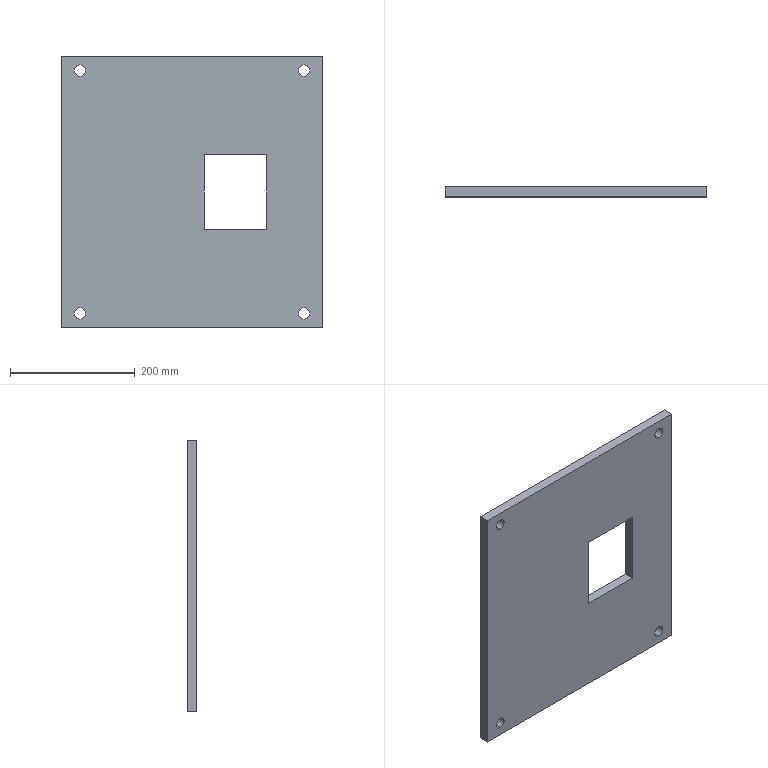Part | STEP file | 01-Base plate 1 | 1 solid | 18 faces | box 420 x 16 x 435 mm | volume 2714914 mm3 | plane 10 | cylinder 8 | commonest cylinder face diameters 18 x8
STEP:
#1=CARTESIAN_POINT('',(0.,0.,0.));
#2=DIRECTION('',(0.,0.,1.));
#3=DIRECTION('',(1.,0.,0.));
#4=AXIS2_PLACEMENT_3D('',#1,#2,#3);
#5=CARTESIAN_POINT('',(30.,0.,421.5));
#6=VERTEX_POINT('',#5);
#7=CARTESIAN_POINT('',(30.,16.,421.5));
#8=VERTEX_POINT('',#7);
#9=CARTESIAN_POINT('',(30.,-14.,421.5));
#10=DIRECTION('',(0.,1.,0.));
#11=VECTOR('',#10,1.);
#12=LINE('',#9,#11);
#13=CARTESIAN_POINT('',(30.,-14.,412.5));
#14=DIRECTION('',(0.,1.,0.));
#15=DIRECTION('',(0.,0.,1.));
#16=AXIS2_PLACEMENT_3D('',#13,#14,#15);
#17=CYLINDRICAL_SURFACE('',#16,9.);
#18=CARTESIAN_POINT('',(6.283,0.));
#19=DIRECTION('',(0.,1.));
#20=VECTOR('',#19,1.);
#21=LINE('',#18,#20);
#22=(GEOMETRIC_REPRESENTATION_CONTEXT(2)PARAMETRIC_REPRESENTATION_CONTEXT()REPRESENTATION_CONTEXT('',''));
#23=DEFINITIONAL_REPRESENTATION('',(#21),#22);
#24=PCURVE('',#17,#23);
#25=CARTESIAN_POINT('',(30.,-14.,412.5));
#26=DIRECTION('',(0.,1.,0.));
#27=DIRECTION('',(0.,0.,1.));
#28=AXIS2_PLACEMENT_3D('',#25,#26,#27);
#29=CYLINDRICAL_SURFACE('',#28,9.);
#30=CARTESIAN_POINT('',(0.,0.));
#31=DIRECTION('',(0.,1.));
#32=VECTOR('',#31,1.);
#33=LINE('',#30,#32);
#34=(GEOMETRIC_REPRESENTATION_CONTEXT(2)PARAMETRIC_REPRESENTATION_CONTEXT()REPRESENTATION_CONTEXT('',''));
#35=DEFINITIONAL_REPRESENTATION('',(#33),#34);
#36=PCURVE('',#29,#35);
#37=SURFACE_CURVE('',#12,(#24,#36),.PCURVE_S1.);
#38=EDGE_CURVE('',#6,#8,#37,.T.);
#39=ORIENTED_EDGE('',*,*,#38,.T.);
#40=CARTESIAN_POINT('',(30.,16.,403.5));
#41=VERTEX_POINT('',#40);
#42=CARTESIAN_POINT('',(30.,16.,412.5));
#43=DIRECTION('',(0.,1.,0.));
#44=DIRECTION('',(0.,0.,1.));
#45=AXIS2_PLACEMENT_3D('',#42,#43,#44);
#46=CIRCLE('',#45,9.);
#47=CARTESIAN_POINT('',(0.,30.));
#48=DIRECTION('',(1.,0.));
#49=VECTOR('',#48,1.);
#50=LINE('',#47,#49);
#51=(GEOMETRIC_REPRESENTATION_CONTEXT(2)PARAMETRIC_REPRESENTATION_CONTEXT()REPRESENTATION_CONTEXT('',''));
#52=DEFINITIONAL_REPRESENTATION('',(#50),#51);
#53=PCURVE('',#17,#52);
#54=CARTESIAN_POINT('',(0.,16.,0.));
#55=DIRECTION('',(0.,1.,0.));
#56=DIRECTION('',(0.,0.,1.));
#57=AXIS2_PLACEMENT_3D('',#54,#55,#56);
#58=PLANE('',#57);
#59=CARTESIAN_POINT('',(412.5,30.));
#60=DIRECTION('',(1.,0.));
#61=AXIS2_PLACEMENT_2D('',#59,#60);
#62=CIRCLE('',#61,9.);
#63=(GEOMETRIC_REPRESENTATION_CONTEXT(2)PARAMETRIC_REPRESENTATION_CONTEXT()REPRESENTATION_CONTEXT('',''));
#64=DEFINITIONAL_REPRESENTATION('',(#62),#63);
#65=PCURVE('',#58,#64);
#66=SURFACE_CURVE('',#46,(#53,#65),.PCURVE_S1.);
#67=EDGE_CURVE('',#41,#8,#66,.T.);
#68=ORIENTED_EDGE('',*,*,#67,.F.);
#69=CARTESIAN_POINT('',(30.,0.,403.5));
#70=VERTEX_POINT('',#69);
#71=CARTESIAN_POINT('',(30.,-14.,403.5));
#72=DIRECTION('',(0.,1.,0.));
#73=VECTOR('',#72,1.);
#74=LINE('',#71,#73);
#75=CARTESIAN_POINT('',(3.142,0.));
#76=DIRECTION('',(0.,1.));
#77=VECTOR('',#76,1.);
#78=LINE('',#75,#77);
#79=(GEOMETRIC_REPRESENTATION_CONTEXT(2)PARAMETRIC_REPRESENTATION_CONTEXT()REPRESENTATION_CONTEXT('',''));
#80=DEFINITIONAL_REPRESENTATION('',(#78),#79);
#81=PCURVE('',#17,#80);
#82=CARTESIAN_POINT('',(3.142,0.));
#83=DIRECTION('',(0.,1.));
#84=VECTOR('',#83,1.);
#85=LINE('',#82,#84);
#86=(GEOMETRIC_REPRESENTATION_CONTEXT(2)PARAMETRIC_REPRESENTATION_CONTEXT()REPRESENTATION_CONTEXT('',''));
#87=DEFINITIONAL_REPRESENTATION('',(#85),#86);
#88=PCURVE('',#29,#87);
#89=SURFACE_CURVE('',#74,(#81,#88),.PCURVE_S1.);
#90=EDGE_CURVE('',#70,#41,#89,.T.);
#91=ORIENTED_EDGE('',*,*,#90,.F.);
#92=CARTESIAN_POINT('',(30.,0.,412.5));
#93=DIRECTION('',(0.,1.,0.));
#94=DIRECTION('',(0.,0.,1.));
#95=AXIS2_PLACEMENT_3D('',#92,#93,#94);
#96=CIRCLE('',#95,9.);
#97=CARTESIAN_POINT('',(0.,14.));
#98=DIRECTION('',(1.,0.));
#99=VECTOR('',#98,1.);
#100=LINE('',#97,#99);
#101=(GEOMETRIC_REPRESENTATION_CONTEXT(2)PARAMETRIC_REPRESENTATION_CONTEXT()REPRESENTATION_CONTEXT('',''));
#102=DEFINITIONAL_REPRESENTATION('',(#100),#101);
#103=PCURVE('',#17,#102);
#104=CARTESIAN_POINT('',(0.,0.,0.));
#105=DIRECTION('',(0.,1.,0.));
#106=DIRECTION('',(0.,0.,1.));
#107=AXIS2_PLACEMENT_3D('',#104,#105,#106);
#108=PLANE('',#107);
#109=CARTESIAN_POINT('',(412.5,30.));
#110=DIRECTION('',(1.,0.));
#111=AXIS2_PLACEMENT_2D('',#109,#110);
#112=CIRCLE('',#111,9.);
#113=(GEOMETRIC_REPRESENTATION_CONTEXT(2)PARAMETRIC_REPRESENTATION_CONTEXT()REPRESENTATION_CONTEXT('',''));
#114=DEFINITIONAL_REPRESENTATION('',(#112),#113);
#115=PCURVE('',#108,#114);
#116=SURFACE_CURVE('',#96,(#103,#115),.PCURVE_S1.);
#117=EDGE_CURVE('',#70,#6,#116,.T.);
#118=ORIENTED_EDGE('',*,*,#117,.T.);
#119=EDGE_LOOP('',(#39,#68,#91,#118));
#120=FACE_BOUND('',#119,.F.);
#121=ADVANCED_FACE('',(#120),#17,.F.);
#122=CARTESIAN_POINT('',(390.,0.,421.5));
#123=VERTEX_POINT('',#122);
#124=CARTESIAN_POINT('',(390.,16.,421.5));
#125=VERTEX_POINT('',#124);
#126=CARTESIAN_POINT('',(390.,-14.,421.5));
#127=DIRECTION('',(0.,1.,0.));
#128=VECTOR('',#127,1.);
#129=LINE('',#126,#128);
#130=CARTESIAN_POINT('',(390.,-14.,412.5));
#131=DIRECTION('',(0.,1.,0.));
#132=DIRECTION('',(0.,0.,1.));
#133=AXIS2_PLACEMENT_3D('',#130,#131,#132);
#134=CYLINDRICAL_SURFACE('',#133,9.);
#135=CARTESIAN_POINT('',(6.283,0.));
#136=DIRECTION('',(0.,1.));
#137=VECTOR('',#136,1.);
#138=LINE('',#135,#137);
#139=(GEOMETRIC_REPRESENTATION_CONTEXT(2)PARAMETRIC_REPRESENTATION_CONTEXT()REPRESENTATION_CONTEXT('',''));
#140=DEFINITIONAL_REPRESENTATION('',(#138),#139);
#141=PCURVE('',#134,#140);
#142=CARTESIAN_POINT('',(390.,-14.,412.5));
#143=DIRECTION('',(0.,1.,0.));
#144=DIRECTION('',(0.,0.,1.));
#145=AXIS2_PLACEMENT_3D('',#142,#143,#144);
#146=CYLINDRICAL_SURFACE('',#145,9.);
#147=CARTESIAN_POINT('',(0.,0.));
#148=DIRECTION('',(0.,1.));
#149=VECTOR('',#148,1.);
#150=LINE('',#147,#149);
#151=(GEOMETRIC_REPRESENTATION_CONTEXT(2)PARAMETRIC_REPRESENTATION_CONTEXT()REPRESENTATION_CONTEXT('',''));
#152=DEFINITIONAL_REPRESENTATION('',(#150),#151);
#153=PCURVE('',#146,#152);
#154=SURFACE_CURVE('',#129,(#141,#153),.PCURVE_S1.);
#155=EDGE_CURVE('',#123,#125,#154,.T.);
#156=ORIENTED_EDGE('',*,*,#155,.T.);
#157=CARTESIAN_POINT('',(390.,16.,403.5));
#158=VERTEX_POINT('',#157);
#159=CARTESIAN_POINT('',(390.,16.,412.5));
#160=DIRECTION('',(0.,1.,0.));
#161=DIRECTION('',(0.,0.,1.));
#162=AXIS2_PLACEMENT_3D('',#159,#160,#161);
#163=CIRCLE('',#162,9.);
#164=CARTESIAN_POINT('',(0.,30.));
#165=DIRECTION('',(1.,0.));
#166=VECTOR('',#165,1.);
#167=LINE('',#164,#166);
#168=(GEOMETRIC_REPRESENTATION_CONTEXT(2)PARAMETRIC_REPRESENTATION_CONTEXT()REPRESENTATION_CONTEXT('',''));
#169=DEFINITIONAL_REPRESENTATION('',(#167),#168);
#170=PCURVE('',#134,#169);
#171=CARTESIAN_POINT('',(412.5,390.));
#172=DIRECTION('',(1.,0.));
#173=AXIS2_PLACEMENT_2D('',#171,#172);
#174=CIRCLE('',#173,9.);
#175=(GEOMETRIC_REPRESENTATION_CONTEXT(2)PARAMETRIC_REPRESENTATION_CONTEXT()REPRESENTATION_CONTEXT('',''));
#176=DEFINITIONAL_REPRESENTATION('',(#174),#175);
#177=PCURVE('',#58,#176);
#178=SURFACE_CURVE('',#163,(#170,#177),.PCURVE_S1.);
#179=EDGE_CURVE('',#158,#125,#178,.T.);
#180=ORIENTED_EDGE('',*,*,#179,.F.);
#181=CARTESIAN_POINT('',(390.,0.,403.5));
#182=VERTEX_POINT('',#181);
#183=CARTESIAN_POINT('',(390.,-14.,403.5));
#184=DIRECTION('',(0.,1.,0.));
#185=VECTOR('',#184,1.);
#186=LINE('',#183,#185);
#187=CARTESIAN_POINT('',(3.142,0.));
#188=DIRECTION('',(0.,1.));
#189=VECTOR('',#188,1.);
#190=LINE('',#187,#189);
#191=(GEOMETRIC_REPRESENTATION_CONTEXT(2)PARAMETRIC_REPRESENTATION_CONTEXT()REPRESENTATION_CONTEXT('',''));
#192=DEFINITIONAL_REPRESENTATION('',(#190),#191);
#193=PCURVE('',#134,#192);
#194=CARTESIAN_POINT('',(3.142,0.));
#195=DIRECTION('',(0.,1.));
#196=VECTOR('',#195,1.);
#197=LINE('',#194,#196);
#198=(GEOMETRIC_REPRESENTATION_CONTEXT(2)PARAMETRIC_REPRESENTATION_CONTEXT()REPRESENTATION_CONTEXT('',''));
#199=DEFINITIONAL_REPRESENTATION('',(#197),#198);
#200=PCURVE('',#146,#199);
#201=SURFACE_CURVE('',#186,(#193,#200),.PCURVE_S1.);
#202=EDGE_CURVE('',#182,#158,#201,.T.);
#203=ORIENTED_EDGE('',*,*,#202,.F.);
#204=CARTESIAN_POINT('',(390.,0.,412.5));
#205=DIRECTION('',(0.,1.,0.));
#206=DIRECTION('',(0.,0.,1.));
#207=AXIS2_PLACEMENT_3D('',#204,#205,#206);
#208=CIRCLE('',#207,9.);
#209=CARTESIAN_POINT('',(0.,14.));
#210=DIRECTION('',(1.,0.));
#211=VECTOR('',#210,1.);
#212=LINE('',#209,#211);
#213=(GEOMETRIC_REPRESENTATION_CONTEXT(2)PARAMETRIC_REPRESENTATION_CONTEXT()REPRESENTATION_CONTEXT('',''));
#214=DEFINITIONAL_REPRESENTATION('',(#212),#213);
#215=PCURVE('',#134,#214);
#216=CARTESIAN_POINT('',(412.5,390.));
#217=DIRECTION('',(1.,0.));
#218=AXIS2_PLACEMENT_2D('',#216,#217);
#219=CIRCLE('',#218,9.);
#220=(GEOMETRIC_REPRESENTATION_CONTEXT(2)PARAMETRIC_REPRESENTATION_CONTEXT()REPRESENTATION_CONTEXT('',''));
#221=DEFINITIONAL_REPRESENTATION('',(#219),#220);
#222=PCURVE('',#108,#221);
#223=SURFACE_CURVE('',#208,(#215,#222),.PCURVE_S1.);
#224=EDGE_CURVE('',#182,#123,#223,.T.);
#225=ORIENTED_EDGE('',*,*,#224,.T.);
#226=EDGE_LOOP('',(#156,#180,#203,#225));
#227=FACE_BOUND('',#226,.F.);
#228=ADVANCED_FACE('',(#227),#134,.F.);
#229=CARTESIAN_POINT('',(390.,0.,31.5));
#230=VERTEX_POINT('',#229);
#231=CARTESIAN_POINT('',(390.,16.,31.5));
#232=VERTEX_POINT('',#231);
#233=CARTESIAN_POINT('',(390.,-14.,31.5));
#234=DIRECTION('',(0.,1.,0.));
#235=VECTOR('',#234,1.);
#236=LINE('',#233,#235);
#237=CARTESIAN_POINT('',(390.,-14.,22.5));
#238=DIRECTION('',(0.,1.,0.));
#239=DIRECTION('',(0.,0.,1.));
#240=AXIS2_PLACEMENT_3D('',#237,#238,#239);
#241=CYLINDRICAL_SURFACE('',#240,9.);
#242=CARTESIAN_POINT('',(6.283,0.));
#243=DIRECTION('',(0.,1.));
#244=VECTOR('',#243,1.);
#245=LINE('',#242,#244);
#246=(GEOMETRIC_REPRESENTATION_CONTEXT(2)PARAMETRIC_REPRESENTATION_CONTEXT()REPRESENTATION_CONTEXT('',''));
#247=DEFINITIONAL_REPRESENTATION('',(#245),#246);
#248=PCURVE('',#241,#247);
#249=CARTESIAN_POINT('',(390.,-14.,22.5));
#250=DIRECTION('',(0.,1.,0.));
#251=DIRECTION('',(0.,0.,1.));
#252=AXIS2_PLACEMENT_3D('',#249,#250,#251);
#253=CYLINDRICAL_SURFACE('',#252,9.);
#254=CARTESIAN_POINT('',(0.,0.));
#255=DIRECTION('',(0.,1.));
#256=VECTOR('',#255,1.);
#257=LINE('',#254,#256);
#258=(GEOMETRIC_REPRESENTATION_CONTEXT(2)PARAMETRIC_REPRESENTATION_CONTEXT()REPRESENTATION_CONTEXT('',''));
#259=DEFINITIONAL_REPRESENTATION('',(#257),#258);
#260=PCURVE('',#253,#259);
#261=SURFACE_CURVE('',#236,(#248,#260),.PCURVE_S1.);
#262=EDGE_CURVE('',#230,#232,#261,.T.);
#263=ORIENTED_EDGE('',*,*,#262,.T.);
#264=CARTESIAN_POINT('',(390.,16.,13.5));
#265=VERTEX_POINT('',#264);
#266=CARTESIAN_POINT('',(390.,16.,22.5));
#267=DIRECTION('',(0.,1.,0.));
#268=DIRECTION('',(0.,0.,1.));
#269=AXIS2_PLACEMENT_3D('',#266,#267,#268);
#270=CIRCLE('',#269,9.);
#271=CARTESIAN_POINT('',(0.,30.));
#272=DIRECTION('',(1.,0.));
#273=VECTOR('',#272,1.);
#274=LINE('',#271,#273);
#275=(GEOMETRIC_REPRESENTATION_CONTEXT(2)PARAMETRIC_REPRESENTATION_CONTEXT()REPRESENTATION_CONTEXT('',''));
#276=DEFINITIONAL_REPRESENTATION('',(#274),#275);
#277=PCURVE('',#241,#276);
#278=CARTESIAN_POINT('',(22.5,390.));
#279=DIRECTION('',(1.,0.));
#280=AXIS2_PLACEMENT_2D('',#278,#279);
#281=CIRCLE('',#280,9.);
#282=(GEOMETRIC_REPRESENTATION_CONTEXT(2)PARAMETRIC_REPRESENTATION_CONTEXT()REPRESENTATION_CONTEXT('',''));
#283=DEFINITIONAL_REPRESENTATION('',(#281),#282);
#284=PCURVE('',#58,#283);
#285=SURFACE_CURVE('',#270,(#277,#284),.PCURVE_S1.);
#286=EDGE_CURVE('',#265,#232,#285,.T.);
#287=ORIENTED_EDGE('',*,*,#286,.F.);
#288=CARTESIAN_POINT('',(390.,0.,13.5));
#289=VERTEX_POINT('',#288);
#290=CARTESIAN_POINT('',(390.,-14.,13.5));
#291=DIRECTION('',(0.,1.,0.));
#292=VECTOR('',#291,1.);
#293=LINE('',#290,#292);
#294=CARTESIAN_POINT('',(3.142,0.));
#295=DIRECTION('',(0.,1.));
#296=VECTOR('',#295,1.);
#297=LINE('',#294,#296);
#298=(GEOMETRIC_REPRESENTATION_CONTEXT(2)PARAMETRIC_REPRESENTATION_CONTEXT()REPRESENTATION_CONTEXT('',''));
#299=DEFINITIONAL_REPRESENTATION('',(#297),#298);
#300=PCURVE('',#241,#299);
#301=CARTESIAN_POINT('',(3.142,0.));
#302=DIRECTION('',(0.,1.));
#303=VECTOR('',#302,1.);
#304=LINE('',#301,#303);
#305=(GEOMETRIC_REPRESENTATION_CONTEXT(2)PARAMETRIC_REPRESENTATION_CONTEXT()REPRESENTATION_CONTEXT('',''));
#306=DEFINITIONAL_REPRESENTATION('',(#304),#305);
#307=PCURVE('',#253,#306);
#308=SURFACE_CURVE('',#293,(#300,#307),.PCURVE_S1.);
#309=EDGE_CURVE('',#289,#265,#308,.T.);
#310=ORIENTED_EDGE('',*,*,#309,.F.);
#311=CARTESIAN_POINT('',(390.,0.,22.5));
#312=DIRECTION('',(0.,1.,0.));
#313=DIRECTION('',(0.,0.,1.));
#314=AXIS2_PLACEMENT_3D('',#311,#312,#313);
#315=CIRCLE('',#314,9.);
#316=CARTESIAN_POINT('',(0.,14.));
#317=DIRECTION('',(1.,0.));
#318=VECTOR('',#317,1.);
#319=LINE('',#316,#318);
#320=(GEOMETRIC_REPRESENTATION_CONTEXT(2)PARAMETRIC_REPRESENTATION_CONTEXT()REPRESENTATION_CONTEXT('',''));
#321=DEFINITIONAL_REPRESENTATION('',(#319),#320);
#322=PCURVE('',#241,#321);
#323=CARTESIAN_POINT('',(22.5,390.));
#324=DIRECTION('',(1.,0.));
#325=AXIS2_PLACEMENT_2D('',#323,#324);
#326=CIRCLE('',#325,9.);
#327=(GEOMETRIC_REPRESENTATION_CONTEXT(2)PARAMETRIC_REPRESENTATION_CONTEXT()REPRESENTATION_CONTEXT('',''));
#328=DEFINITIONAL_REPRESENTATION('',(#326),#327);
#329=PCURVE('',#108,#328);
#330=SURFACE_CURVE('',#315,(#322,#329),.PCURVE_S1.);
#331=EDGE_CURVE('',#289,#230,#330,.T.);
#332=ORIENTED_EDGE('',*,*,#331,.T.);
#333=EDGE_LOOP('',(#263,#287,#310,#332));
#334=FACE_BOUND('',#333,.F.);
#335=ADVANCED_FACE('',(#334),#241,.F.);
#336=CARTESIAN_POINT('',(30.,0.,31.5));
#337=VERTEX_POINT('',#336);
#338=CARTESIAN_POINT('',(30.,16.,31.5));
#339=VERTEX_POINT('',#338);
#340=CARTESIAN_POINT('',(30.,-14.,31.5));
#341=DIRECTION('',(0.,1.,0.));
#342=VECTOR('',#341,1.);
#343=LINE('',#340,#342);
#344=CARTESIAN_POINT('',(30.,-14.,22.5));
#345=DIRECTION('',(0.,1.,0.));
#346=DIRECTION('',(0.,0.,1.));
#347=AXIS2_PLACEMENT_3D('',#344,#345,#346);
#348=CYLINDRICAL_SURFACE('',#347,9.);
#349=CARTESIAN_POINT('',(6.283,0.));
#350=DIRECTION('',(0.,1.));
#351=VECTOR('',#350,1.);
#352=LINE('',#349,#351);
#353=(GEOMETRIC_REPRESENTATION_CONTEXT(2)PARAMETRIC_REPRESENTATION_CONTEXT()REPRESENTATION_CONTEXT('',''));
#354=DEFINITIONAL_REPRESENTATION('',(#352),#353);
#355=PCURVE('',#348,#354);
#356=CARTESIAN_POINT('',(30.,-14.,22.5));
#357=DIRECTION('',(0.,1.,0.));
#358=DIRECTION('',(0.,0.,1.));
#359=AXIS2_PLACEMENT_3D('',#356,#357,#358);
#360=CYLINDRICAL_SURFACE('',#359,9.);
#361=CARTESIAN_POINT('',(0.,0.));
#362=DIRECTION('',(0.,1.));
#363=VECTOR('',#362,1.);
#364=LINE('',#361,#363);
#365=(GEOMETRIC_REPRESENTATION_CONTEXT(2)PARAMETRIC_REPRESENTATION_CONTEXT()REPRESENTATION_CONTEXT('',''));
#366=DEFINITIONAL_REPRESENTATION('',(#364),#365);
#367=PCURVE('',#360,#366);
#368=SURFACE_CURVE('',#343,(#355,#367),.PCURVE_S1.);
#369=EDGE_CURVE('',#337,#339,#368,.T.);
#370=ORIENTED_EDGE('',*,*,#369,.T.);
#371=CARTESIAN_POINT('',(30.,16.,13.5));
#372=VERTEX_POINT('',#371);
#373=CARTESIAN_POINT('',(30.,16.,22.5));
#374=DIRECTION('',(0.,1.,0.));
#375=DIRECTION('',(0.,0.,1.));
#376=AXIS2_PLACEMENT_3D('',#373,#374,#375);
#377=CIRCLE('',#376,9.);
#378=CARTESIAN_POINT('',(0.,30.));
#379=DIRECTION('',(1.,0.));
#380=VECTOR('',#379,1.);
#381=LINE('',#378,#380);
#382=(GEOMETRIC_REPRESENTATION_CONTEXT(2)PARAMETRIC_REPRESENTATION_CONTEXT()REPRESENTATION_CONTEXT('',''));
#383=DEFINITIONAL_REPRESENTATION('',(#381),#382);
#384=PCURVE('',#348,#383);
#385=CARTESIAN_POINT('',(22.5,30.));
#386=DIRECTION('',(1.,0.));
#387=AXIS2_PLACEMENT_2D('',#385,#386);
#388=CIRCLE('',#387,9.);
#389=(GEOMETRIC_REPRESENTATION_CONTEXT(2)PARAMETRIC_REPRESENTATION_CONTEXT()REPRESENTATION_CONTEXT('',''));
#390=DEFINITIONAL_REPRESENTATION('',(#388),#389);
#391=PCURVE('',#58,#390);
#392=SURFACE_CURVE('',#377,(#384,#391),.PCURVE_S1.);
#393=EDGE_CURVE('',#372,#339,#392,.T.);
#394=ORIENTED_EDGE('',*,*,#393,.F.);
#395=CARTESIAN_POINT('',(30.,0.,13.5));
#396=VERTEX_POINT('',#395);
#397=CARTESIAN_POINT('',(30.,-14.,13.5));
#398=DIRECTION('',(0.,1.,0.));
#399=VECTOR('',#398,1.);
#400=LINE('',#397,#399);
#401=CARTESIAN_POINT('',(3.142,0.));
#402=DIRECTION('',(0.,1.));
#403=VECTOR('',#402,1.);
#404=LINE('',#401,#403);
#405=(GEOMETRIC_REPRESENTATION_CONTEXT(2)PARAMETRIC_REPRESENTATION_CONTEXT()REPRESENTATION_CONTEXT('',''));
#406=DEFINITIONAL_REPRESENTATION('',(#404),#405);
#407=PCURVE('',#348,#406);
#408=CARTESIAN_POINT('',(3.142,0.));
#409=DIRECTION('',(0.,1.));
#410=VECTOR('',#409,1.);
#411=LINE('',#408,#410);
#412=(GEOMETRIC_REPRESENTATION_CONTEXT(2)PARAMETRIC_REPRESENTATION_CONTEXT()REPRESENTATION_CONTEXT('',''));
#413=DEFINITIONAL_REPRESENTATION('',(#411),#412);
#414=PCURVE('',#360,#413);
#415=SURFACE_CURVE('',#400,(#407,#414),.PCURVE_S1.);
#416=EDGE_CURVE('',#396,#372,#415,.T.);
#417=ORIENTED_EDGE('',*,*,#416,.F.);
#418=CARTESIAN_POINT('',(30.,0.,22.5));
#419=DIRECTION('',(0.,1.,0.));
#420=DIRECTION('',(0.,0.,1.));
#421=AXIS2_PLACEMENT_3D('',#418,#419,#420);
#422=CIRCLE('',#421,9.);
#423=CARTESIAN_POINT('',(0.,14.));
#424=DIRECTION('',(1.,0.));
#425=VECTOR('',#424,1.);
#426=LINE('',#423,#425);
#427=(GEOMETRIC_REPRESENTATION_CONTEXT(2)PARAMETRIC_REPRESENTATION_CONTEXT()REPRESENTATION_CONTEXT('',''));
#428=DEFINITIONAL_REPRESENTATION('',(#426),#427);
#429=PCURVE('',#348,#428);
#430=CARTESIAN_POINT('',(22.5,30.));
#431=DIRECTION('',(1.,0.));
#432=AXIS2_PLACEMENT_2D('',#430,#431);
#433=CIRCLE('',#432,9.);
#434=(GEOMETRIC_REPRESENTATION_CONTEXT(2)PARAMETRIC_REPRESENTATION_CONTEXT()REPRESENTATION_CONTEXT('',''));
#435=DEFINITIONAL_REPRESENTATION('',(#433),#434);
#436=PCURVE('',#108,#435);
#437=SURFACE_CURVE('',#422,(#429,#436),.PCURVE_S1.);
#438=EDGE_CURVE('',#396,#337,#437,.T.);
#439=ORIENTED_EDGE('',*,*,#438,.T.);
#440=EDGE_LOOP('',(#370,#394,#417,#439));
#441=FACE_BOUND('',#440,.F.);
#442=ADVANCED_FACE('',(#441),#348,.F.);
#443=CARTESIAN_POINT('',(0.,0.,0.));
#444=VERTEX_POINT('',#443);
#445=CARTESIAN_POINT('',(0.,0.,435.));
#446=VERTEX_POINT('',#445);
#447=CARTESIAN_POINT('',(0.,0.,0.));
#448=DIRECTION('',(0.,0.,1.));
#449=VECTOR('',#448,1.);
#450=LINE('',#447,#449);
#451=CARTESIAN_POINT('',(0.,16.,0.));
#452=DIRECTION('',(1.,0.,0.));
#453=DIRECTION('',(0.,0.,-1.));
#454=AXIS2_PLACEMENT_3D('',#451,#452,#453);
#455=PLANE('',#454);
#456=CARTESIAN_POINT('',(0.,-16.));
#457=DIRECTION('',(-1.,0.));
#458=VECTOR('',#457,1.);
#459=LINE('',#456,#458);
#460=(GEOMETRIC_REPRESENTATION_CONTEXT(2)PARAMETRIC_REPRESENTATION_CONTEXT()REPRESENTATION_CONTEXT('',''));
#461=DEFINITIONAL_REPRESENTATION('',(#459),#460);
#462=PCURVE('',#455,#461);
#463=CARTESIAN_POINT('',(0.,0.));
#464=DIRECTION('',(1.,0.));
#465=VECTOR('',#464,1.);
#466=LINE('',#463,#465);
#467=(GEOMETRIC_REPRESENTATION_CONTEXT(2)PARAMETRIC_REPRESENTATION_CONTEXT()REPRESENTATION_CONTEXT('',''));
#468=DEFINITIONAL_REPRESENTATION('',(#466),#467);
#469=PCURVE('',#108,#468);
#470=SURFACE_CURVE('',#450,(#462,#469),.PCURVE_S1.);
#471=EDGE_CURVE('',#444,#446,#470,.T.);
#472=ORIENTED_EDGE('',*,*,#471,.T.);
#473=CARTESIAN_POINT('',(0.,16.,435.));
#474=VERTEX_POINT('',#473);
#475=CARTESIAN_POINT('',(0.,16.,435.));
#476=DIRECTION('',(0.,-1.,0.));
#477=VECTOR('',#476,1.);
#478=LINE('',#475,#477);
#479=CARTESIAN_POINT('',(-435.,0.));
#480=DIRECTION('',(0.,-1.));
#481=VECTOR('',#480,1.);
#482=LINE('',#479,#481);
#483=(GEOMETRIC_REPRESENTATION_CONTEXT(2)PARAMETRIC_REPRESENTATION_CONTEXT()REPRESENTATION_CONTEXT('',''));
#484=DEFINITIONAL_REPRESENTATION('',(#482),#483);
#485=PCURVE('',#455,#484);
#486=CARTESIAN_POINT('',(0.,16.,435.));
#487=DIRECTION('',(0.,0.,-1.));
#488=DIRECTION('',(-1.,0.,0.));
#489=AXIS2_PLACEMENT_3D('',#486,#487,#488);
#490=PLANE('',#489);
#491=CARTESIAN_POINT('',(0.,0.));
#492=DIRECTION('',(0.,-1.));
#493=VECTOR('',#492,1.);
#494=LINE('',#491,#493);
#495=(GEOMETRIC_REPRESENTATION_CONTEXT(2)PARAMETRIC_REPRESENTATION_CONTEXT()REPRESENTATION_CONTEXT('',''));
#496=DEFINITIONAL_REPRESENTATION('',(#494),#495);
#497=PCURVE('',#490,#496);
#498=SURFACE_CURVE('',#478,(#485,#497),.PCURVE_S1.);
#499=EDGE_CURVE('',#474,#446,#498,.T.);
#500=ORIENTED_EDGE('',*,*,#499,.F.);
#501=CARTESIAN_POINT('',(0.,16.,0.));
#502=VERTEX_POINT('',#501);
#503=CARTESIAN_POINT('',(0.,16.,0.));
#504=DIRECTION('',(0.,0.,1.));
#505=VECTOR('',#504,1.);
#506=LINE('',#503,#505);
#507=CARTESIAN_POINT('',(0.,0.));
#508=DIRECTION('',(-1.,0.));
#509=VECTOR('',#508,1.);
#510=LINE('',#507,#509);
#511=(GEOMETRIC_REPRESENTATION_CONTEXT(2)PARAMETRIC_REPRESENTATION_CONTEXT()REPRESENTATION_CONTEXT('',''));
#512=DEFINITIONAL_REPRESENTATION('',(#510),#511);
#513=PCURVE('',#455,#512);
#514=CARTESIAN_POINT('',(0.,0.));
#515=DIRECTION('',(1.,0.));
#516=VECTOR('',#515,1.);
#517=LINE('',#514,#516);
#518=(GEOMETRIC_REPRESENTATION_CONTEXT(2)PARAMETRIC_REPRESENTATION_CONTEXT()REPRESENTATION_CONTEXT('',''));
#519=DEFINITIONAL_REPRESENTATION('',(#517),#518);
#520=PCURVE('',#58,#519);
#521=SURFACE_CURVE('',#506,(#513,#520),.PCURVE_S1.);
#522=EDGE_CURVE('',#502,#474,#521,.T.);
#523=ORIENTED_EDGE('',*,*,#522,.F.);
#524=CARTESIAN_POINT('',(0.,16.,0.));
#525=DIRECTION('',(0.,-1.,0.));
#526=VECTOR('',#525,1.);
#527=LINE('',#524,#526);
#528=CARTESIAN_POINT('',(0.,0.));
#529=DIRECTION('',(0.,-1.));
#530=VECTOR('',#529,1.);
#531=LINE('',#528,#530);
#532=(GEOMETRIC_REPRESENTATION_CONTEXT(2)PARAMETRIC_REPRESENTATION_CONTEXT()REPRESENTATION_CONTEXT('',''));
#533=DEFINITIONAL_REPRESENTATION('',(#531),#532);
#534=PCURVE('',#455,#533);
#535=CARTESIAN_POINT('',(0.,16.,0.));
#536=DIRECTION('',(0.,0.,1.));
#537=DIRECTION('',(1.,0.,0.));
#538=AXIS2_PLACEMENT_3D('',#535,#536,#537);
#539=PLANE('',#538);
#540=CARTESIAN_POINT('',(0.,0.));
#541=DIRECTION('',(0.,-1.));
#542=VECTOR('',#541,1.);
#543=LINE('',#540,#542);
#544=(GEOMETRIC_REPRESENTATION_CONTEXT(2)PARAMETRIC_REPRESENTATION_CONTEXT()REPRESENTATION_CONTEXT('',''));
#545=DEFINITIONAL_REPRESENTATION('',(#543),#544);
#546=PCURVE('',#539,#545);
#547=SURFACE_CURVE('',#527,(#534,#546),.PCURVE_S1.);
#548=EDGE_CURVE('',#502,#444,#547,.T.);
#549=ORIENTED_EDGE('',*,*,#548,.T.);
#550=EDGE_LOOP('',(#472,#500,#523,#549));
#551=FACE_BOUND('',#550,.T.);
#552=ADVANCED_FACE('',(#551),#455,.F.);
#553=CARTESIAN_POINT('',(420.,0.,435.));
#554=VERTEX_POINT('',#553);
#555=CARTESIAN_POINT('',(0.,0.,435.));
#556=DIRECTION('',(1.,0.,0.));
#557=VECTOR('',#556,1.);
#558=LINE('',#555,#557);
#559=CARTESIAN_POINT('',(0.,-16.));
#560=DIRECTION('',(-1.,0.));
#561=VECTOR('',#560,1.);
#562=LINE('',#559,#561);
#563=(GEOMETRIC_REPRESENTATION_CONTEXT(2)PARAMETRIC_REPRESENTATION_CONTEXT()REPRESENTATION_CONTEXT('',''));
#564=DEFINITIONAL_REPRESENTATION('',(#562),#563);
#565=PCURVE('',#490,#564);
#566=CARTESIAN_POINT('',(435.,0.));
#567=DIRECTION('',(0.,1.));
#568=VECTOR('',#567,1.);
#569=LINE('',#566,#568);
#570=(GEOMETRIC_REPRESENTATION_CONTEXT(2)PARAMETRIC_REPRESENTATION_CONTEXT()REPRESENTATION_CONTEXT('',''));
#571=DEFINITIONAL_REPRESENTATION('',(#569),#570);
#572=PCURVE('',#108,#571);
#573=SURFACE_CURVE('',#558,(#565,#572),.PCURVE_S1.);
#574=EDGE_CURVE('',#446,#554,#573,.T.);
#575=ORIENTED_EDGE('',*,*,#574,.T.);
#576=CARTESIAN_POINT('',(420.,16.,435.));
#577=VERTEX_POINT('',#576);
#578=CARTESIAN_POINT('',(420.,16.,435.));
#579=DIRECTION('',(0.,-1.,0.));
#580=VECTOR('',#579,1.);
#581=LINE('',#578,#580);
#582=CARTESIAN_POINT('',(-420.,0.));
#583=DIRECTION('',(0.,-1.));
#584=VECTOR('',#583,1.);
#585=LINE('',#582,#584);
#586=(GEOMETRIC_REPRESENTATION_CONTEXT(2)PARAMETRIC_REPRESENTATION_CONTEXT()REPRESENTATION_CONTEXT('',''));
#587=DEFINITIONAL_REPRESENTATION('',(#585),#586);
#588=PCURVE('',#490,#587);
#589=CARTESIAN_POINT('',(420.,16.,0.));
#590=DIRECTION('',(-1.,0.,0.));
#591=DIRECTION('',(0.,0.,1.));
#592=AXIS2_PLACEMENT_3D('',#589,#590,#591);
#593=PLANE('',#592);
#594=CARTESIAN_POINT('',(435.,0.));
#595=DIRECTION('',(0.,-1.));
#596=VECTOR('',#595,1.);
#597=LINE('',#594,#596);
#598=(GEOMETRIC_REPRESENTATION_CONTEXT(2)PARAMETRIC_REPRESENTATION_CONTEXT()REPRESENTATION_CONTEXT('',''));
#599=DEFINITIONAL_REPRESENTATION('',(#597),#598);
#600=PCURVE('',#593,#599);
#601=SURFACE_CURVE('',#581,(#588,#600),.PCURVE_S1.);
#602=EDGE_CURVE('',#577,#554,#601,.T.);
#603=ORIENTED_EDGE('',*,*,#602,.F.);
#604=CARTESIAN_POINT('',(0.,16.,435.));
#605=DIRECTION('',(1.,0.,0.));
#606=VECTOR('',#605,1.);
#607=LINE('',#604,#606);
#608=CARTESIAN_POINT('',(0.,0.));
#609=DIRECTION('',(-1.,0.));
#610=VECTOR('',#609,1.);
#611=LINE('',#608,#610);
#612=(GEOMETRIC_REPRESENTATION_CONTEXT(2)PARAMETRIC_REPRESENTATION_CONTEXT()REPRESENTATION_CONTEXT('',''));
#613=DEFINITIONAL_REPRESENTATION('',(#611),#612);
#614=PCURVE('',#490,#613);
#615=CARTESIAN_POINT('',(435.,0.));
#616=DIRECTION('',(0.,1.));
#617=VECTOR('',#616,1.);
#618=LINE('',#615,#617);
#619=(GEOMETRIC_REPRESENTATION_CONTEXT(2)PARAMETRIC_REPRESENTATION_CONTEXT()REPRESENTATION_CONTEXT('',''));
#620=DEFINITIONAL_REPRESENTATION('',(#618),#619);
#621=PCURVE('',#58,#620);
#622=SURFACE_CURVE('',#607,(#614,#621),.PCURVE_S1.);
#623=EDGE_CURVE('',#474,#577,#622,.T.);
#624=ORIENTED_EDGE('',*,*,#623,.F.);
#625=ORIENTED_EDGE('',*,*,#499,.T.);
#626=EDGE_LOOP('',(#575,#603,#624,#625));
#627=FACE_BOUND('',#626,.T.);
#628=ADVANCED_FACE('',(#627),#490,.F.);
#629=CARTESIAN_POINT('',(420.,0.,0.));
#630=VERTEX_POINT('',#629);
#631=CARTESIAN_POINT('',(420.,0.,0.));
#632=DIRECTION('',(0.,0.,-1.));
#633=VECTOR('',#632,1.);
#634=LINE('',#631,#633);
#635=CARTESIAN_POINT('',(0.,-16.));
#636=DIRECTION('',(-1.,0.));
#637=VECTOR('',#636,1.);
#638=LINE('',#635,#637);
#639=(GEOMETRIC_REPRESENTATION_CONTEXT(2)PARAMETRIC_REPRESENTATION_CONTEXT()REPRESENTATION_CONTEXT('',''));
#640=DEFINITIONAL_REPRESENTATION('',(#638),#639);
#641=PCURVE('',#593,#640);
#642=CARTESIAN_POINT('',(0.,420.));
#643=DIRECTION('',(-1.,0.));
#644=VECTOR('',#643,1.);
#645=LINE('',#642,#644);
#646=(GEOMETRIC_REPRESENTATION_CONTEXT(2)PARAMETRIC_REPRESENTATION_CONTEXT()REPRESENTATION_CONTEXT('',''));
#647=DEFINITIONAL_REPRESENTATION('',(#645),#646);
#648=PCURVE('',#108,#647);
#649=SURFACE_CURVE('',#634,(#641,#648),.PCURVE_S1.);
#650=EDGE_CURVE('',#554,#630,#649,.T.);
#651=ORIENTED_EDGE('',*,*,#650,.T.);
#652=CARTESIAN_POINT('',(420.,16.,0.));
#653=VERTEX_POINT('',#652);
#654=CARTESIAN_POINT('',(420.,16.,0.));
#655=DIRECTION('',(0.,-1.,0.));
#656=VECTOR('',#655,1.);
#657=LINE('',#654,#656);
#658=CARTESIAN_POINT('',(0.,0.));
#659=DIRECTION('',(0.,-1.));
#660=VECTOR('',#659,1.);
#661=LINE('',#658,#660);
#662=(GEOMETRIC_REPRESENTATION_CONTEXT(2)PARAMETRIC_REPRESENTATION_CONTEXT()REPRESENTATION_CONTEXT('',''));
#663=DEFINITIONAL_REPRESENTATION('',(#661),#662);
#664=PCURVE('',#593,#663);
#665=CARTESIAN_POINT('',(420.,0.));
#666=DIRECTION('',(0.,-1.));
#667=VECTOR('',#666,1.);
#668=LINE('',#665,#667);
#669=(GEOMETRIC_REPRESENTATION_CONTEXT(2)PARAMETRIC_REPRESENTATION_CONTEXT()REPRESENTATION_CONTEXT('',''));
#670=DEFINITIONAL_REPRESENTATION('',(#668),#669);
#671=PCURVE('',#539,#670);
#672=SURFACE_CURVE('',#657,(#664,#671),.PCURVE_S1.);
#673=EDGE_CURVE('',#653,#630,#672,.T.);
#674=ORIENTED_EDGE('',*,*,#673,.F.);
#675=CARTESIAN_POINT('',(420.,16.,0.));
#676=DIRECTION('',(0.,0.,-1.));
#677=VECTOR('',#676,1.);
#678=LINE('',#675,#677);
#679=CARTESIAN_POINT('',(0.,0.));
#680=DIRECTION('',(-1.,0.));
#681=VECTOR('',#680,1.);
#682=LINE('',#679,#681);
#683=(GEOMETRIC_REPRESENTATION_CONTEXT(2)PARAMETRIC_REPRESENTATION_CONTEXT()REPRESENTATION_CONTEXT('',''));
#684=DEFINITIONAL_REPRESENTATION('',(#682),#683);
#685=PCURVE('',#593,#684);
#686=CARTESIAN_POINT('',(0.,420.));
#687=DIRECTION('',(-1.,0.));
#688=VECTOR('',#687,1.);
#689=LINE('',#686,#688);
#690=(GEOMETRIC_REPRESENTATION_CONTEXT(2)PARAMETRIC_REPRESENTATION_CONTEXT()REPRESENTATION_CONTEXT('',''));
#691=DEFINITIONAL_REPRESENTATION('',(#689),#690);
#692=PCURVE('',#58,#691);
#693=SURFACE_CURVE('',#678,(#685,#692),.PCURVE_S1.);
#694=EDGE_CURVE('',#577,#653,#693,.T.);
#695=ORIENTED_EDGE('',*,*,#694,.F.);
#696=ORIENTED_EDGE('',*,*,#602,.T.);
#697=EDGE_LOOP('',(#651,#674,#695,#696));
#698=FACE_BOUND('',#697,.T.);
#699=ADVANCED_FACE('',(#698),#593,.F.);
#700=CARTESIAN_POINT('',(0.,0.,0.));
#701=DIRECTION('',(-1.,0.,0.));
#702=VECTOR('',#701,1.);
#703=LINE('',#700,#702);
#704=CARTESIAN_POINT('',(0.,-16.));
#705=DIRECTION('',(-1.,0.));
#706=VECTOR('',#705,1.);
#707=LINE('',#704,#706);
#708=(GEOMETRIC_REPRESENTATION_CONTEXT(2)PARAMETRIC_REPRESENTATION_CONTEXT()REPRESENTATION_CONTEXT('',''));
#709=DEFINITIONAL_REPRESENTATION('',(#707),#708);
#710=PCURVE('',#539,#709);
#711=CARTESIAN_POINT('',(0.,0.));
#712=DIRECTION('',(0.,-1.));
#713=VECTOR('',#712,1.);
#714=LINE('',#711,#713);
#715=(GEOMETRIC_REPRESENTATION_CONTEXT(2)PARAMETRIC_REPRESENTATION_CONTEXT()REPRESENTATION_CONTEXT('',''));
#716=DEFINITIONAL_REPRESENTATION('',(#714),#715);
#717=PCURVE('',#108,#716);
#718=SURFACE_CURVE('',#703,(#710,#717),.PCURVE_S1.);
#719=EDGE_CURVE('',#630,#444,#718,.T.);
#720=ORIENTED_EDGE('',*,*,#719,.T.);
#721=ORIENTED_EDGE('',*,*,#548,.F.);
#722=CARTESIAN_POINT('',(0.,16.,0.));
#723=DIRECTION('',(-1.,0.,0.));
#724=VECTOR('',#723,1.);
#725=LINE('',#722,#724);
#726=CARTESIAN_POINT('',(0.,0.));
#727=DIRECTION('',(-1.,0.));
#728=VECTOR('',#727,1.);
#729=LINE('',#726,#728);
#730=(GEOMETRIC_REPRESENTATION_CONTEXT(2)PARAMETRIC_REPRESENTATION_CONTEXT()REPRESENTATION_CONTEXT('',''));
#731=DEFINITIONAL_REPRESENTATION('',(#729),#730);
#732=PCURVE('',#539,#731);
#733=CARTESIAN_POINT('',(0.,0.));
#734=DIRECTION('',(0.,-1.));
#735=VECTOR('',#734,1.);
#736=LINE('',#733,#735);
#737=(GEOMETRIC_REPRESENTATION_CONTEXT(2)PARAMETRIC_REPRESENTATION_CONTEXT()REPRESENTATION_CONTEXT('',''));
#738=DEFINITIONAL_REPRESENTATION('',(#736),#737);
#739=PCURVE('',#58,#738);
#740=SURFACE_CURVE('',#725,(#732,#739),.PCURVE_S1.);
#741=EDGE_CURVE('',#653,#502,#740,.T.);
#742=ORIENTED_EDGE('',*,*,#741,.F.);
#743=ORIENTED_EDGE('',*,*,#673,.T.);
#744=EDGE_LOOP('',(#720,#721,#742,#743));
#745=FACE_BOUND('',#744,.T.);
#746=ADVANCED_FACE('',(#745),#539,.F.);
#747=CARTESIAN_POINT('',(230.,16.,157.5));
#748=VERTEX_POINT('',#747);
#749=CARTESIAN_POINT('',(230.,16.,277.5));
#750=VERTEX_POINT('',#749);
#751=CARTESIAN_POINT('',(230.,16.,157.5));
#752=DIRECTION('',(0.,0.,1.));
#753=VECTOR('',#752,1.);
#754=LINE('',#751,#753);
#755=CARTESIAN_POINT('',(157.5,230.));
#756=DIRECTION('',(1.,0.));
#757=VECTOR('',#756,1.);
#758=LINE('',#755,#757);
#759=(GEOMETRIC_REPRESENTATION_CONTEXT(2)PARAMETRIC_REPRESENTATION_CONTEXT()REPRESENTATION_CONTEXT('',''));
#760=DEFINITIONAL_REPRESENTATION('',(#758),#759);
#761=PCURVE('',#58,#760);
#762=CARTESIAN_POINT('',(230.,-4.,157.5));
#763=DIRECTION('',(-1.,0.,0.));
#764=DIRECTION('',(0.,0.,1.));
#765=AXIS2_PLACEMENT_3D('',#762,#763,#764);
#766=PLANE('',#765);
#767=CARTESIAN_POINT('',(0.,20.));
#768=DIRECTION('',(1.,0.));
#769=VECTOR('',#768,1.);
#770=LINE('',#767,#769);
#771=(GEOMETRIC_REPRESENTATION_CONTEXT(2)PARAMETRIC_REPRESENTATION_CONTEXT()REPRESENTATION_CONTEXT('',''));
#772=DEFINITIONAL_REPRESENTATION('',(#770),#771);
#773=PCURVE('',#766,#772);
#774=SURFACE_CURVE('',#754,(#761,#773),.PCURVE_S1.);
#775=EDGE_CURVE('',#748,#750,#774,.T.);
#776=ORIENTED_EDGE('',*,*,#775,.F.);
#777=CARTESIAN_POINT('',(330.,16.,157.5));
#778=VERTEX_POINT('',#777);
#779=CARTESIAN_POINT('',(230.,16.,157.5));
#780=DIRECTION('',(-1.,0.,0.));
#781=VECTOR('',#780,1.);
#782=LINE('',#779,#781);
#783=CARTESIAN_POINT('',(157.5,230.));
#784=DIRECTION('',(0.,-1.));
#785=VECTOR('',#784,1.);
#786=LINE('',#783,#785);
#787=(GEOMETRIC_REPRESENTATION_CONTEXT(2)PARAMETRIC_REPRESENTATION_CONTEXT()REPRESENTATION_CONTEXT('',''));
#788=DEFINITIONAL_REPRESENTATION('',(#786),#787);
#789=PCURVE('',#58,#788);
#790=CARTESIAN_POINT('',(230.,-4.,157.5));
#791=DIRECTION('',(0.,0.,-1.));
#792=DIRECTION('',(-1.,0.,0.));
#793=AXIS2_PLACEMENT_3D('',#790,#791,#792);
#794=PLANE('',#793);
#795=CARTESIAN_POINT('',(0.,20.));
#796=DIRECTION('',(1.,0.));
#797=VECTOR('',#796,1.);
#798=LINE('',#795,#797);
#799=(GEOMETRIC_REPRESENTATION_CONTEXT(2)PARAMETRIC_REPRESENTATION_CONTEXT()REPRESENTATION_CONTEXT('',''));
#800=DEFINITIONAL_REPRESENTATION('',(#798),#799);
#801=PCURVE('',#794,#800);
#802=SURFACE_CURVE('',#782,(#789,#801),.PCURVE_S1.);
#803=EDGE_CURVE('',#778,#748,#802,.T.);
#804=ORIENTED_EDGE('',*,*,#803,.F.);
#805=CARTESIAN_POINT('',(330.,16.,277.5));
#806=VERTEX_POINT('',#805);
#807=CARTESIAN_POINT('',(330.,16.,157.5));
#808=DIRECTION('',(0.,0.,-1.));
#809=VECTOR('',#808,1.);
#810=LINE('',#807,#809);
#811=CARTESIAN_POINT('',(157.5,330.));
#812=DIRECTION('',(-1.,0.));
#813=VECTOR('',#812,1.);
#814=LINE('',#811,#813);
#815=(GEOMETRIC_REPRESENTATION_CONTEXT(2)PARAMETRIC_REPRESENTATION_CONTEXT()REPRESENTATION_CONTEXT('',''));
#816=DEFINITIONAL_REPRESENTATION('',(#814),#815);
#817=PCURVE('',#58,#816);
#818=CARTESIAN_POINT('',(330.,-4.,157.5));
#819=DIRECTION('',(1.,0.,0.));
#820=DIRECTION('',(0.,0.,-1.));
#821=AXIS2_PLACEMENT_3D('',#818,#819,#820);
#822=PLANE('',#821);
#823=CARTESIAN_POINT('',(0.,20.));
#824=DIRECTION('',(1.,0.));
#825=VECTOR('',#824,1.);
#826=LINE('',#823,#825);
#827=(GEOMETRIC_REPRESENTATION_CONTEXT(2)PARAMETRIC_REPRESENTATION_CONTEXT()REPRESENTATION_CONTEXT('',''));
#828=DEFINITIONAL_REPRESENTATION('',(#826),#827);
#829=PCURVE('',#822,#828);
#830=SURFACE_CURVE('',#810,(#817,#829),.PCURVE_S1.);
#831=EDGE_CURVE('',#806,#778,#830,.T.);
#832=ORIENTED_EDGE('',*,*,#831,.F.);
#833=CARTESIAN_POINT('',(230.,16.,277.5));
#834=DIRECTION('',(1.,0.,0.));
#835=VECTOR('',#834,1.);
#836=LINE('',#833,#835);
#837=CARTESIAN_POINT('',(277.5,230.));
#838=DIRECTION('',(0.,1.));
#839=VECTOR('',#838,1.);
#840=LINE('',#837,#839);
#841=(GEOMETRIC_REPRESENTATION_CONTEXT(2)PARAMETRIC_REPRESENTATION_CONTEXT()REPRESENTATION_CONTEXT('',''));
#842=DEFINITIONAL_REPRESENTATION('',(#840),#841);
#843=PCURVE('',#58,#842);
#844=CARTESIAN_POINT('',(230.,-4.,277.5));
#845=DIRECTION('',(0.,0.,1.));
#846=DIRECTION('',(1.,0.,0.));
#847=AXIS2_PLACEMENT_3D('',#844,#845,#846);
#848=PLANE('',#847);
#849=CARTESIAN_POINT('',(0.,20.));
#850=DIRECTION('',(1.,0.));
#851=VECTOR('',#850,1.);
#852=LINE('',#849,#851);
#853=(GEOMETRIC_REPRESENTATION_CONTEXT(2)PARAMETRIC_REPRESENTATION_CONTEXT()REPRESENTATION_CONTEXT('',''));
#854=DEFINITIONAL_REPRESENTATION('',(#852),#853);
#855=PCURVE('',#848,#854);
#856=SURFACE_CURVE('',#836,(#843,#855),.PCURVE_S1.);
#857=EDGE_CURVE('',#750,#806,#856,.T.);
#858=ORIENTED_EDGE('',*,*,#857,.F.);
#859=EDGE_LOOP('',(#776,#804,#832,#858));
#860=FACE_BOUND('',#859,.T.);
#861=CARTESIAN_POINT('',(30.,16.,412.5));
#862=DIRECTION('',(0.,1.,0.));
#863=DIRECTION('',(0.,0.,1.));
#864=AXIS2_PLACEMENT_3D('',#861,#862,#863);
#865=CIRCLE('',#864,9.);
#866=CARTESIAN_POINT('',(412.5,30.));
#867=DIRECTION('',(1.,0.));
#868=AXIS2_PLACEMENT_2D('',#866,#867);
#869=CIRCLE('',#868,9.);
#870=(GEOMETRIC_REPRESENTATION_CONTEXT(2)PARAMETRIC_REPRESENTATION_CONTEXT()REPRESENTATION_CONTEXT('',''));
#871=DEFINITIONAL_REPRESENTATION('',(#869),#870);
#872=PCURVE('',#58,#871);
#873=CARTESIAN_POINT('',(0.,30.));
#874=DIRECTION('',(1.,0.));
#875=VECTOR('',#874,1.);
#876=LINE('',#873,#875);
#877=(GEOMETRIC_REPRESENTATION_CONTEXT(2)PARAMETRIC_REPRESENTATION_CONTEXT()REPRESENTATION_CONTEXT('',''));
#878=DEFINITIONAL_REPRESENTATION('',(#876),#877);
#879=PCURVE('',#29,#878);
#880=SURFACE_CURVE('',#865,(#872,#879),.PCURVE_S1.);
#881=EDGE_CURVE('',#8,#41,#880,.T.);
#882=ORIENTED_EDGE('',*,*,#881,.F.);
#883=ORIENTED_EDGE('',*,*,#67,.F.);
#884=EDGE_LOOP('',(#882,#883));
#885=FACE_BOUND('',#884,.T.);
#886=CARTESIAN_POINT('',(390.,16.,412.5));
#887=DIRECTION('',(0.,1.,0.));
#888=DIRECTION('',(0.,0.,1.));
#889=AXIS2_PLACEMENT_3D('',#886,#887,#888);
#890=CIRCLE('',#889,9.);
#891=CARTESIAN_POINT('',(412.5,390.));
#892=DIRECTION('',(1.,0.));
#893=AXIS2_PLACEMENT_2D('',#891,#892);
#894=CIRCLE('',#893,9.);
#895=(GEOMETRIC_REPRESENTATION_CONTEXT(2)PARAMETRIC_REPRESENTATION_CONTEXT()REPRESENTATION_CONTEXT('',''));
#896=DEFINITIONAL_REPRESENTATION('',(#894),#895);
#897=PCURVE('',#58,#896);
#898=CARTESIAN_POINT('',(0.,30.));
#899=DIRECTION('',(1.,0.));
#900=VECTOR('',#899,1.);
#901=LINE('',#898,#900);
#902=(GEOMETRIC_REPRESENTATION_CONTEXT(2)PARAMETRIC_REPRESENTATION_CONTEXT()REPRESENTATION_CONTEXT('',''));
#903=DEFINITIONAL_REPRESENTATION('',(#901),#902);
#904=PCURVE('',#146,#903);
#905=SURFACE_CURVE('',#890,(#897,#904),.PCURVE_S1.);
#906=EDGE_CURVE('',#125,#158,#905,.T.);
#907=ORIENTED_EDGE('',*,*,#906,.F.);
#908=ORIENTED_EDGE('',*,*,#179,.F.);
#909=EDGE_LOOP('',(#907,#908));
#910=FACE_BOUND('',#909,.T.);
#911=CARTESIAN_POINT('',(390.,16.,22.5));
#912=DIRECTION('',(0.,1.,0.));
#913=DIRECTION('',(0.,0.,1.));
#914=AXIS2_PLACEMENT_3D('',#911,#912,#913);
#915=CIRCLE('',#914,9.);
#916=CARTESIAN_POINT('',(22.5,390.));
#917=DIRECTION('',(1.,0.));
#918=AXIS2_PLACEMENT_2D('',#916,#917);
#919=CIRCLE('',#918,9.);
#920=(GEOMETRIC_REPRESENTATION_CONTEXT(2)PARAMETRIC_REPRESENTATION_CONTEXT()REPRESENTATION_CONTEXT('',''));
#921=DEFINITIONAL_REPRESENTATION('',(#919),#920);
#922=PCURVE('',#58,#921);
#923=CARTESIAN_POINT('',(0.,30.));
#924=DIRECTION('',(1.,0.));
#925=VECTOR('',#924,1.);
#926=LINE('',#923,#925);
#927=(GEOMETRIC_REPRESENTATION_CONTEXT(2)PARAMETRIC_REPRESENTATION_CONTEXT()REPRESENTATION_CONTEXT('',''));
#928=DEFINITIONAL_REPRESENTATION('',(#926),#927);
#929=PCURVE('',#253,#928);
#930=SURFACE_CURVE('',#915,(#922,#929),.PCURVE_S1.);
#931=EDGE_CURVE('',#232,#265,#930,.T.);
#932=ORIENTED_EDGE('',*,*,#931,.F.);
#933=ORIENTED_EDGE('',*,*,#286,.F.);
#934=EDGE_LOOP('',(#932,#933));
#935=FACE_BOUND('',#934,.T.);
#936=CARTESIAN_POINT('',(30.,16.,22.5));
#937=DIRECTION('',(0.,1.,0.));
#938=DIRECTION('',(0.,0.,1.));
#939=AXIS2_PLACEMENT_3D('',#936,#937,#938);
#940=CIRCLE('',#939,9.);
#941=CARTESIAN_POINT('',(22.5,30.));
#942=DIRECTION('',(1.,0.));
#943=AXIS2_PLACEMENT_2D('',#941,#942);
#944=CIRCLE('',#943,9.);
#945=(GEOMETRIC_REPRESENTATION_CONTEXT(2)PARAMETRIC_REPRESENTATION_CONTEXT()REPRESENTATION_CONTEXT('',''));
#946=DEFINITIONAL_REPRESENTATION('',(#944),#945);
#947=PCURVE('',#58,#946);
#948=CARTESIAN_POINT('',(0.,30.));
#949=DIRECTION('',(1.,0.));
#950=VECTOR('',#949,1.);
#951=LINE('',#948,#950);
#952=(GEOMETRIC_REPRESENTATION_CONTEXT(2)PARAMETRIC_REPRESENTATION_CONTEXT()REPRESENTATION_CONTEXT('',''));
#953=DEFINITIONAL_REPRESENTATION('',(#951),#952);
#954=PCURVE('',#360,#953);
#955=SURFACE_CURVE('',#940,(#947,#954),.PCURVE_S1.);
#956=EDGE_CURVE('',#339,#372,#955,.T.);
#957=ORIENTED_EDGE('',*,*,#956,.F.);
#958=ORIENTED_EDGE('',*,*,#393,.F.);
#959=EDGE_LOOP('',(#957,#958));
#960=FACE_BOUND('',#959,.T.);
#961=ORIENTED_EDGE('',*,*,#522,.T.);
#962=ORIENTED_EDGE('',*,*,#623,.T.);
#963=ORIENTED_EDGE('',*,*,#694,.T.);
#964=ORIENTED_EDGE('',*,*,#741,.T.);
#965=EDGE_LOOP('',(#961,#962,#963,#964));
#966=FACE_BOUND('',#965,.T.);
#967=ADVANCED_FACE('',(#860,#885,#910,#935,#960,#966),#58,.T.);
#968=CARTESIAN_POINT('',(330.,0.,157.5));
#969=VERTEX_POINT('',#968);
#970=CARTESIAN_POINT('',(230.,0.,157.5));
#971=VERTEX_POINT('',#970);
#972=CARTESIAN_POINT('',(0.,0.,157.5));
#973=DIRECTION('',(-1.,0.,0.));
#974=VECTOR('',#973,1.);
#975=LINE('',#972,#974);
#976=CARTESIAN_POINT('',(157.5,0.));
#977=DIRECTION('',(0.,-1.));
#978=VECTOR('',#977,1.);
#979=LINE('',#976,#978);
#980=(GEOMETRIC_REPRESENTATION_CONTEXT(2)PARAMETRIC_REPRESENTATION_CONTEXT()REPRESENTATION_CONTEXT('',''));
#981=DEFINITIONAL_REPRESENTATION('',(#979),#980);
#982=PCURVE('',#108,#981);
#983=CARTESIAN_POINT('',(230.,4.));
#984=DIRECTION('',(1.,0.));
#985=VECTOR('',#984,1.);
#986=LINE('',#983,#985);
#987=(GEOMETRIC_REPRESENTATION_CONTEXT(2)PARAMETRIC_REPRESENTATION_CONTEXT()REPRESENTATION_CONTEXT('',''));
#988=DEFINITIONAL_REPRESENTATION('',(#986),#987);
#989=PCURVE('',#794,#988);
#990=SURFACE_CURVE('',#975,(#982,#989),.PCURVE_S1.);
#991=EDGE_CURVE('',#969,#971,#990,.T.);
#992=ORIENTED_EDGE('',*,*,#991,.T.);
#993=CARTESIAN_POINT('',(230.,0.,277.5));
#994=VERTEX_POINT('',#993);
#995=CARTESIAN_POINT('',(230.,0.,0.));
#996=DIRECTION('',(0.,0.,1.));
#997=VECTOR('',#996,1.);
#998=LINE('',#995,#997);
#999=CARTESIAN_POINT('',(0.,230.));
#1000=DIRECTION('',(1.,0.));
#1001=VECTOR('',#1000,1.);
#1002=LINE('',#999,#1001);
#1003=(GEOMETRIC_REPRESENTATION_CONTEXT(2)PARAMETRIC_REPRESENTATION_CONTEXT()REPRESENTATION_CONTEXT('',''));
#1004=DEFINITIONAL_REPRESENTATION('',(#1002),#1003);
#1005=PCURVE('',#108,#1004);
#1006=CARTESIAN_POINT('',(-157.5,4.));
#1007=DIRECTION('',(1.,0.));
#1008=VECTOR('',#1007,1.);
#1009=LINE('',#1006,#1008);
#1010=(GEOMETRIC_REPRESENTATION_CONTEXT(2)PARAMETRIC_REPRESENTATION_CONTEXT()REPRESENTATION_CONTEXT('',''));
#1011=DEFINITIONAL_REPRESENTATION('',(#1009),#1010);
#1012=PCURVE('',#766,#1011);
#1013=SURFACE_CURVE('',#998,(#1005,#1012),.PCURVE_S1.);
#1014=EDGE_CURVE('',#971,#994,#1013,.T.);
#1015=ORIENTED_EDGE('',*,*,#1014,.T.);
#1016=CARTESIAN_POINT('',(330.,0.,277.5));
#1017=VERTEX_POINT('',#1016);
#1018=CARTESIAN_POINT('',(0.,0.,277.5));
#1019=DIRECTION('',(1.,0.,0.));
#1020=VECTOR('',#1019,1.);
#1021=LINE('',#1018,#1020);
#1022=CARTESIAN_POINT('',(277.5,0.));
#1023=DIRECTION('',(0.,1.));
#1024=VECTOR('',#1023,1.);
#1025=LINE('',#1022,#1024);
#1026=(GEOMETRIC_REPRESENTATION_CONTEXT(2)PARAMETRIC_REPRESENTATION_CONTEXT()REPRESENTATION_CONTEXT('',''));
#1027=DEFINITIONAL_REPRESENTATION('',(#1025),#1026);
#1028=PCURVE('',#108,#1027);
#1029=CARTESIAN_POINT('',(-230.,4.));
#1030=DIRECTION('',(1.,0.));
#1031=VECTOR('',#1030,1.);
#1032=LINE('',#1029,#1031);
#1033=(GEOMETRIC_REPRESENTATION_CONTEXT(2)PARAMETRIC_REPRESENTATION_CONTEXT()REPRESENTATION_CONTEXT('',''));
#1034=DEFINITIONAL_REPRESENTATION('',(#1032),#1033);
#1035=PCURVE('',#848,#1034);
#1036=SURFACE_CURVE('',#1021,(#1028,#1035),.PCURVE_S1.);
#1037=EDGE_CURVE('',#994,#1017,#1036,.T.);
#1038=ORIENTED_EDGE('',*,*,#1037,.T.);
#1039=CARTESIAN_POINT('',(330.,0.,0.));
#1040=DIRECTION('',(0.,0.,-1.));
#1041=VECTOR('',#1040,1.);
#1042=LINE('',#1039,#1041);
#1043=CARTESIAN_POINT('',(0.,330.));
#1044=DIRECTION('',(-1.,0.));
#1045=VECTOR('',#1044,1.);
#1046=LINE('',#1043,#1045);
#1047=(GEOMETRIC_REPRESENTATION_CONTEXT(2)PARAMETRIC_REPRESENTATION_CONTEXT()REPRESENTATION_CONTEXT('',''));
#1048=DEFINITIONAL_REPRESENTATION('',(#1046),#1047);
#1049=PCURVE('',#108,#1048);
#1050=CARTESIAN_POINT('',(157.5,4.));
#1051=DIRECTION('',(1.,0.));
#1052=VECTOR('',#1051,1.);
#1053=LINE('',#1050,#1052);
#1054=(GEOMETRIC_REPRESENTATION_CONTEXT(2)PARAMETRIC_REPRESENTATION_CONTEXT()REPRESENTATION_CONTEXT('',''));
#1055=DEFINITIONAL_REPRESENTATION('',(#1053),#1054);
#1056=PCURVE('',#822,#1055);
#1057=SURFACE_CURVE('',#1042,(#1049,#1056),.PCURVE_S1.);
#1058=EDGE_CURVE('',#1017,#969,#1057,.T.);
#1059=ORIENTED_EDGE('',*,*,#1058,.T.);
#1060=EDGE_LOOP('',(#992,#1015,#1038,#1059));
#1061=FACE_BOUND('',#1060,.T.);
#1062=CARTESIAN_POINT('',(30.,0.,412.5));
#1063=DIRECTION('',(0.,1.,0.));
#1064=DIRECTION('',(0.,0.,1.));
#1065=AXIS2_PLACEMENT_3D('',#1062,#1063,#1064);
#1066=CIRCLE('',#1065,9.);
#1067=CARTESIAN_POINT('',(412.5,30.));
#1068=DIRECTION('',(1.,0.));
#1069=AXIS2_PLACEMENT_2D('',#1067,#1068);
#1070=CIRCLE('',#1069,9.);
#1071=(GEOMETRIC_REPRESENTATION_CONTEXT(2)PARAMETRIC_REPRESENTATION_CONTEXT()REPRESENTATION_CONTEXT('',''));
#1072=DEFINITIONAL_REPRESENTATION('',(#1070),#1071);
#1073=PCURVE('',#108,#1072);
#1074=CARTESIAN_POINT('',(0.,14.));
#1075=DIRECTION('',(1.,0.));
#1076=VECTOR('',#1075,1.);
#1077=LINE('',#1074,#1076);
#1078=(GEOMETRIC_REPRESENTATION_CONTEXT(2)PARAMETRIC_REPRESENTATION_CONTEXT()REPRESENTATION_CONTEXT('',''));
#1079=DEFINITIONAL_REPRESENTATION('',(#1077),#1078);
#1080=PCURVE('',#29,#1079);
#1081=SURFACE_CURVE('',#1066,(#1073,#1080),.PCURVE_S1.);
#1082=EDGE_CURVE('',#6,#70,#1081,.T.);
#1083=ORIENTED_EDGE('',*,*,#1082,.T.);
#1084=ORIENTED_EDGE('',*,*,#117,.T.);
#1085=EDGE_LOOP('',(#1083,#1084));
#1086=FACE_BOUND('',#1085,.T.);
#1087=CARTESIAN_POINT('',(390.,0.,412.5));
#1088=DIRECTION('',(0.,1.,0.));
#1089=DIRECTION('',(0.,0.,1.));
#1090=AXIS2_PLACEMENT_3D('',#1087,#1088,#1089);
#1091=CIRCLE('',#1090,9.);
#1092=CARTESIAN_POINT('',(412.5,390.));
#1093=DIRECTION('',(1.,0.));
#1094=AXIS2_PLACEMENT_2D('',#1092,#1093);
#1095=CIRCLE('',#1094,9.);
#1096=(GEOMETRIC_REPRESENTATION_CONTEXT(2)PARAMETRIC_REPRESENTATION_CONTEXT()REPRESENTATION_CONTEXT('',''));
#1097=DEFINITIONAL_REPRESENTATION('',(#1095),#1096);
#1098=PCURVE('',#108,#1097);
#1099=CARTESIAN_POINT('',(0.,14.));
#1100=DIRECTION('',(1.,0.));
#1101=VECTOR('',#1100,1.);
#1102=LINE('',#1099,#1101);
#1103=(GEOMETRIC_REPRESENTATION_CONTEXT(2)PARAMETRIC_REPRESENTATION_CONTEXT()REPRESENTATION_CONTEXT('',''));
#1104=DEFINITIONAL_REPRESENTATION('',(#1102),#1103);
#1105=PCURVE('',#146,#1104);
#1106=SURFACE_CURVE('',#1091,(#1098,#1105),.PCURVE_S1.);
#1107=EDGE_CURVE('',#123,#182,#1106,.T.);
#1108=ORIENTED_EDGE('',*,*,#1107,.T.);
#1109=ORIENTED_EDGE('',*,*,#224,.T.);
#1110=EDGE_LOOP('',(#1108,#1109));
#1111=FACE_BOUND('',#1110,.T.);
#1112=CARTESIAN_POINT('',(390.,0.,22.5));
#1113=DIRECTION('',(0.,1.,0.));
#1114=DIRECTION('',(0.,0.,1.));
#1115=AXIS2_PLACEMENT_3D('',#1112,#1113,#1114);
#1116=CIRCLE('',#1115,9.);
#1117=CARTESIAN_POINT('',(22.5,390.));
#1118=DIRECTION('',(1.,0.));
#1119=AXIS2_PLACEMENT_2D('',#1117,#1118);
#1120=CIRCLE('',#1119,9.);
#1121=(GEOMETRIC_REPRESENTATION_CONTEXT(2)PARAMETRIC_REPRESENTATION_CONTEXT()REPRESENTATION_CONTEXT('',''));
#1122=DEFINITIONAL_REPRESENTATION('',(#1120),#1121);
#1123=PCURVE('',#108,#1122);
#1124=CARTESIAN_POINT('',(0.,14.));
#1125=DIRECTION('',(1.,0.));
#1126=VECTOR('',#1125,1.);
#1127=LINE('',#1124,#1126);
#1128=(GEOMETRIC_REPRESENTATION_CONTEXT(2)PARAMETRIC_REPRESENTATION_CONTEXT()REPRESENTATION_CONTEXT('',''));
#1129=DEFINITIONAL_REPRESENTATION('',(#1127),#1128);
#1130=PCURVE('',#253,#1129);
#1131=SURFACE_CURVE('',#1116,(#1123,#1130),.PCURVE_S1.);
#1132=EDGE_CURVE('',#230,#289,#1131,.T.);
#1133=ORIENTED_EDGE('',*,*,#1132,.T.);
#1134=ORIENTED_EDGE('',*,*,#331,.T.);
#1135=EDGE_LOOP('',(#1133,#1134));
#1136=FACE_BOUND('',#1135,.T.);
#1137=CARTESIAN_POINT('',(30.,0.,22.5));
#1138=DIRECTION('',(0.,1.,0.));
#1139=DIRECTION('',(0.,0.,1.));
#1140=AXIS2_PLACEMENT_3D('',#1137,#1138,#1139);
#1141=CIRCLE('',#1140,9.);
#1142=CARTESIAN_POINT('',(22.5,30.));
#1143=DIRECTION('',(1.,0.));
#1144=AXIS2_PLACEMENT_2D('',#1142,#1143);
#1145=CIRCLE('',#1144,9.);
#1146=(GEOMETRIC_REPRESENTATION_CONTEXT(2)PARAMETRIC_REPRESENTATION_CONTEXT()REPRESENTATION_CONTEXT('',''));
#1147=DEFINITIONAL_REPRESENTATION('',(#1145),#1146);
#1148=PCURVE('',#108,#1147);
#1149=CARTESIAN_POINT('',(0.,14.));
#1150=DIRECTION('',(1.,0.));
#1151=VECTOR('',#1150,1.);
#1152=LINE('',#1149,#1151);
#1153=(GEOMETRIC_REPRESENTATION_CONTEXT(2)PARAMETRIC_REPRESENTATION_CONTEXT()REPRESENTATION_CONTEXT('',''));
#1154=DEFINITIONAL_REPRESENTATION('',(#1152),#1153);
#1155=PCURVE('',#360,#1154);
#1156=SURFACE_CURVE('',#1141,(#1148,#1155),.PCURVE_S1.);
#1157=EDGE_CURVE('',#337,#396,#1156,.T.);
#1158=ORIENTED_EDGE('',*,*,#1157,.T.);
#1159=ORIENTED_EDGE('',*,*,#438,.T.);
#1160=EDGE_LOOP('',(#1158,#1159));
#1161=FACE_BOUND('',#1160,.T.);
#1162=ORIENTED_EDGE('',*,*,#471,.F.);
#1163=ORIENTED_EDGE('',*,*,#719,.F.);
#1164=ORIENTED_EDGE('',*,*,#650,.F.);
#1165=ORIENTED_EDGE('',*,*,#574,.F.);
#1166=EDGE_LOOP('',(#1162,#1163,#1164,#1165));
#1167=FACE_BOUND('',#1166,.T.);
#1168=ADVANCED_FACE('',(#1061,#1086,#1111,#1136,#1161,#1167),#108,.F.);
#1169=ORIENTED_EDGE('',*,*,#956,.F.);
#1170=ORIENTED_EDGE('',*,*,#369,.F.);
#1171=ORIENTED_EDGE('',*,*,#1157,.T.);
#1172=ORIENTED_EDGE('',*,*,#416,.T.);
#1173=EDGE_LOOP('',(#1169,#1170,#1171,#1172));
#1174=FACE_BOUND('',#1173,.F.);
#1175=ADVANCED_FACE('',(#1174),#360,.F.);
#1176=ORIENTED_EDGE('',*,*,#931,.F.);
#1177=ORIENTED_EDGE('',*,*,#262,.F.);
#1178=ORIENTED_EDGE('',*,*,#1132,.T.);
#1179=ORIENTED_EDGE('',*,*,#309,.T.);
#1180=EDGE_LOOP('',(#1176,#1177,#1178,#1179));
#1181=FACE_BOUND('',#1180,.F.);
#1182=ADVANCED_FACE('',(#1181),#253,.F.);
#1183=ORIENTED_EDGE('',*,*,#906,.F.);
#1184=ORIENTED_EDGE('',*,*,#155,.F.);
#1185=ORIENTED_EDGE('',*,*,#1107,.T.);
#1186=ORIENTED_EDGE('',*,*,#202,.T.);
#1187=EDGE_LOOP('',(#1183,#1184,#1185,#1186));
#1188=FACE_BOUND('',#1187,.F.);
#1189=ADVANCED_FACE('',(#1188),#146,.F.);
#1190=ORIENTED_EDGE('',*,*,#881,.F.);
#1191=ORIENTED_EDGE('',*,*,#38,.F.);
#1192=ORIENTED_EDGE('',*,*,#1082,.T.);
#1193=ORIENTED_EDGE('',*,*,#90,.T.);
#1194=EDGE_LOOP('',(#1190,#1191,#1192,#1193));
#1195=FACE_BOUND('',#1194,.F.);
#1196=ADVANCED_FACE('',(#1195),#29,.F.);
#1197=CARTESIAN_POINT('',(230.,-4.,157.5));
#1198=DIRECTION('',(0.,1.,0.));
#1199=VECTOR('',#1198,1.);
#1200=LINE('',#1197,#1199);
#1201=CARTESIAN_POINT('',(0.,0.));
#1202=DIRECTION('',(0.,1.));
#1203=VECTOR('',#1202,1.);
#1204=LINE('',#1201,#1203);
#1205=(GEOMETRIC_REPRESENTATION_CONTEXT(2)PARAMETRIC_REPRESENTATION_CONTEXT()REPRESENTATION_CONTEXT('',''));
#1206=DEFINITIONAL_REPRESENTATION('',(#1204),#1205);
#1207=PCURVE('',#766,#1206);
#1208=CARTESIAN_POINT('',(0.,0.));
#1209=DIRECTION('',(0.,1.));
#1210=VECTOR('',#1209,1.);
#1211=LINE('',#1208,#1210);
#1212=(GEOMETRIC_REPRESENTATION_CONTEXT(2)PARAMETRIC_REPRESENTATION_CONTEXT()REPRESENTATION_CONTEXT('',''));
#1213=DEFINITIONAL_REPRESENTATION('',(#1211),#1212);
#1214=PCURVE('',#794,#1213);
#1215=SURFACE_CURVE('',#1200,(#1207,#1214),.PCURVE_S1.);
#1216=EDGE_CURVE('',#971,#748,#1215,.T.);
#1217=ORIENTED_EDGE('',*,*,#1216,.T.);
#1218=ORIENTED_EDGE('',*,*,#775,.T.);
#1219=CARTESIAN_POINT('',(230.,-4.,277.5));
#1220=DIRECTION('',(0.,1.,0.));
#1221=VECTOR('',#1220,1.);
#1222=LINE('',#1219,#1221);
#1223=CARTESIAN_POINT('',(120.,0.));
#1224=DIRECTION('',(0.,1.));
#1225=VECTOR('',#1224,1.);
#1226=LINE('',#1223,#1225);
#1227=(GEOMETRIC_REPRESENTATION_CONTEXT(2)PARAMETRIC_REPRESENTATION_CONTEXT()REPRESENTATION_CONTEXT('',''));
#1228=DEFINITIONAL_REPRESENTATION('',(#1226),#1227);
#1229=PCURVE('',#766,#1228);
#1230=CARTESIAN_POINT('',(0.,0.));
#1231=DIRECTION('',(0.,1.));
#1232=VECTOR('',#1231,1.);
#1233=LINE('',#1230,#1232);
#1234=(GEOMETRIC_REPRESENTATION_CONTEXT(2)PARAMETRIC_REPRESENTATION_CONTEXT()REPRESENTATION_CONTEXT('',''));
#1235=DEFINITIONAL_REPRESENTATION('',(#1233),#1234);
#1236=PCURVE('',#848,#1235);
#1237=SURFACE_CURVE('',#1222,(#1229,#1236),.PCURVE_S1.);
#1238=EDGE_CURVE('',#994,#750,#1237,.T.);
#1239=ORIENTED_EDGE('',*,*,#1238,.F.);
#1240=ORIENTED_EDGE('',*,*,#1014,.F.);
#1241=EDGE_LOOP('',(#1217,#1218,#1239,#1240));
#1242=FACE_BOUND('',#1241,.T.);
#1243=ADVANCED_FACE('',(#1242),#766,.F.);
#1244=CARTESIAN_POINT('',(330.,-4.,157.5));
#1245=DIRECTION('',(0.,1.,0.));
#1246=VECTOR('',#1245,1.);
#1247=LINE('',#1244,#1246);
#1248=CARTESIAN_POINT('',(-100.,0.));
#1249=DIRECTION('',(0.,1.));
#1250=VECTOR('',#1249,1.);
#1251=LINE('',#1248,#1250);
#1252=(GEOMETRIC_REPRESENTATION_CONTEXT(2)PARAMETRIC_REPRESENTATION_CONTEXT()REPRESENTATION_CONTEXT('',''));
#1253=DEFINITIONAL_REPRESENTATION('',(#1251),#1252);
#1254=PCURVE('',#794,#1253);
#1255=CARTESIAN_POINT('',(0.,0.));
#1256=DIRECTION('',(0.,1.));
#1257=VECTOR('',#1256,1.);
#1258=LINE('',#1255,#1257);
#1259=(GEOMETRIC_REPRESENTATION_CONTEXT(2)PARAMETRIC_REPRESENTATION_CONTEXT()REPRESENTATION_CONTEXT('',''));
#1260=DEFINITIONAL_REPRESENTATION('',(#1258),#1259);
#1261=PCURVE('',#822,#1260);
#1262=SURFACE_CURVE('',#1247,(#1254,#1261),.PCURVE_S1.);
#1263=EDGE_CURVE('',#969,#778,#1262,.T.);
#1264=ORIENTED_EDGE('',*,*,#1263,.T.);
#1265=ORIENTED_EDGE('',*,*,#803,.T.);
#1266=ORIENTED_EDGE('',*,*,#1216,.F.);
#1267=ORIENTED_EDGE('',*,*,#991,.F.);
#1268=EDGE_LOOP('',(#1264,#1265,#1266,#1267));
#1269=FACE_BOUND('',#1268,.T.);
#1270=ADVANCED_FACE('',(#1269),#794,.F.);
#1271=CARTESIAN_POINT('',(330.,-4.,277.5));
#1272=DIRECTION('',(0.,1.,0.));
#1273=VECTOR('',#1272,1.);
#1274=LINE('',#1271,#1273);
#1275=CARTESIAN_POINT('',(-120.,0.));
#1276=DIRECTION('',(0.,1.));
#1277=VECTOR('',#1276,1.);
#1278=LINE('',#1275,#1277);
#1279=(GEOMETRIC_REPRESENTATION_CONTEXT(2)PARAMETRIC_REPRESENTATION_CONTEXT()REPRESENTATION_CONTEXT('',''));
#1280=DEFINITIONAL_REPRESENTATION('',(#1278),#1279);
#1281=PCURVE('',#822,#1280);
#1282=CARTESIAN_POINT('',(100.,0.));
#1283=DIRECTION('',(0.,1.));
#1284=VECTOR('',#1283,1.);
#1285=LINE('',#1282,#1284);
#1286=(GEOMETRIC_REPRESENTATION_CONTEXT(2)PARAMETRIC_REPRESENTATION_CONTEXT()REPRESENTATION_CONTEXT('',''));
#1287=DEFINITIONAL_REPRESENTATION('',(#1285),#1286);
#1288=PCURVE('',#848,#1287);
#1289=SURFACE_CURVE('',#1274,(#1281,#1288),.PCURVE_S1.);
#1290=EDGE_CURVE('',#1017,#806,#1289,.T.);
#1291=ORIENTED_EDGE('',*,*,#1290,.T.);
#1292=ORIENTED_EDGE('',*,*,#831,.T.);
#1293=ORIENTED_EDGE('',*,*,#1263,.F.);
#1294=ORIENTED_EDGE('',*,*,#1058,.F.);
#1295=EDGE_LOOP('',(#1291,#1292,#1293,#1294));
#1296=FACE_BOUND('',#1295,.T.);
#1297=ADVANCED_FACE('',(#1296),#822,.F.);
#1298=ORIENTED_EDGE('',*,*,#1238,.T.);
#1299=ORIENTED_EDGE('',*,*,#857,.T.);
#1300=ORIENTED_EDGE('',*,*,#1290,.F.);
#1301=ORIENTED_EDGE('',*,*,#1037,.F.);
#1302=EDGE_LOOP('',(#1298,#1299,#1300,#1301));
#1303=FACE_BOUND('',#1302,.T.);
#1304=ADVANCED_FACE('',(#1303),#848,.F.);
#1305=CLOSED_SHELL('',(#121,#228,#335,#442,#552,#628,#699,#746,#967,#1168,#1175,#1182,#1189,#1196,#1243,#1270,#1297,#1304));
#1306=MANIFOLD_SOLID_BREP('',#1305);
#1307=(LENGTH_UNIT()NAMED_UNIT(*)SI_UNIT(.MILLI.,.METRE.));
#1308=UNCERTAINTY_MEASURE_WITH_UNIT(LENGTH_MEASURE(0.0000001),#1307,'','');
#1309=(NAMED_UNIT(*)PLANE_ANGLE_UNIT()SI_UNIT($,.RADIAN.));
#1310=(NAMED_UNIT(*)SI_UNIT($,.STERADIAN.)SOLID_ANGLE_UNIT());
#1311=(GEOMETRIC_REPRESENTATION_CONTEXT(3)GLOBAL_UNCERTAINTY_ASSIGNED_CONTEXT((#1308))GLOBAL_UNIT_ASSIGNED_CONTEXT((#1307,#1309,#1310))REPRESENTATION_CONTEXT('',''));
#1312=ADVANCED_BREP_SHAPE_REPRESENTATION('',(#4,#1306),#1311);